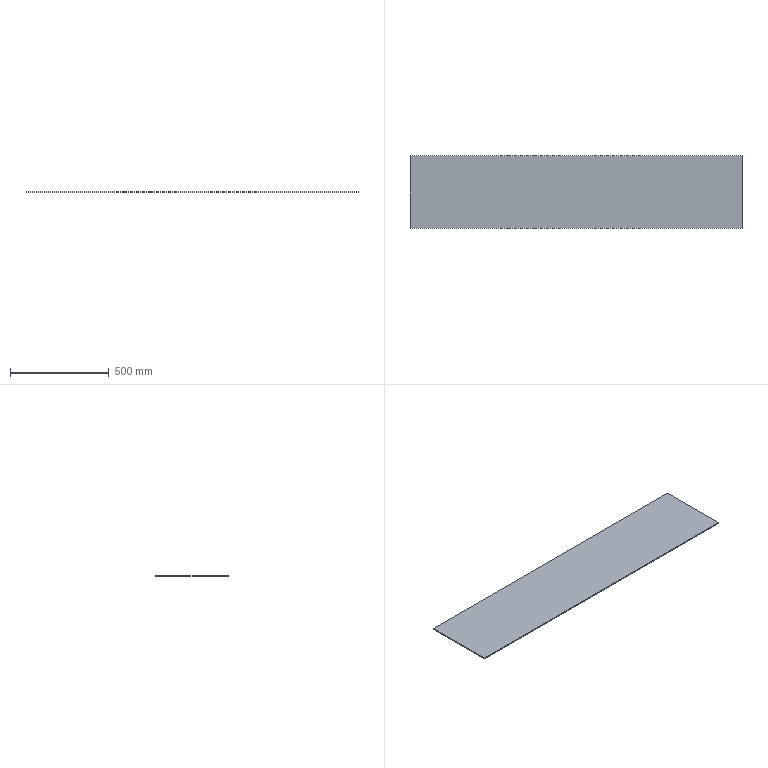Part | SolidWorks | features FlatPattern 1, SMBaseFlange 1, SheetMetal 1 | 1 solid | 6 faces | box 1685 x 367 x 5 mm | volume 3091975 mm3 | plane 6
STEP:
#1=CARTESIAN_POINT('',(842.5,-183.5,0.));
#2=VERTEX_POINT('',#1);
#3=CARTESIAN_POINT('',(842.5,183.5,0.));
#4=VERTEX_POINT('',#3);
#5=CARTESIAN_POINT('',(842.5,183.5,0.));
#6=DIRECTION('',(0.,1.,0.));
#7=VECTOR('',#6,1000.);
#8=LINE('',#5,#7);
#9=EDGE_CURVE('',#2,#4,#8,.T.);
#10=ORIENTED_EDGE('',*,*,#9,.F.);
#11=CARTESIAN_POINT('',(842.5,-183.5,-5.));
#12=VERTEX_POINT('',#11);
#13=CARTESIAN_POINT('',(842.5,-183.5,-5.));
#14=DIRECTION('',(0.,0.,1.));
#15=VECTOR('',#14,1000.);
#16=LINE('',#13,#15);
#17=EDGE_CURVE('',#12,#2,#16,.T.);
#18=ORIENTED_EDGE('',*,*,#17,.F.);
#19=CARTESIAN_POINT('',(842.5,183.5,-5.));
#20=VERTEX_POINT('',#19);
#21=CARTESIAN_POINT('',(842.5,183.5,-5.));
#22=DIRECTION('',(0.,1.,0.));
#23=VECTOR('',#22,1000.);
#24=LINE('',#21,#23);
#25=EDGE_CURVE('',#12,#20,#24,.T.);
#26=ORIENTED_EDGE('',*,*,#25,.T.);
#27=CARTESIAN_POINT('',(842.5,183.5,-5.));
#28=DIRECTION('',(0.,0.,1.));
#29=VECTOR('',#28,1000.);
#30=LINE('',#27,#29);
#31=EDGE_CURVE('',#20,#4,#30,.T.);
#32=ORIENTED_EDGE('',*,*,#31,.T.);
#33=EDGE_LOOP('',(#10,#18,#26,#32));
#34=FACE_OUTER_BOUND('',#33,.T.);
#35=CARTESIAN_POINT('',(842.5,183.5,-5.));
#36=DIRECTION('',(1.,0.,0.));
#37=DIRECTION('',(0.,0.,-1.));
#38=AXIS2_PLACEMENT_3D('',#35,#36,#37);
#39=PLANE('',#38);
#40=ADVANCED_FACE('',(#34),#39,.T.);
#41=CARTESIAN_POINT('',(-842.5,-183.5,0.));
#42=VERTEX_POINT('',#41);
#43=CARTESIAN_POINT('',(-842.5,-183.5,0.));
#44=DIRECTION('',(1.,0.,0.));
#45=VECTOR('',#44,1000.);
#46=LINE('',#43,#45);
#47=EDGE_CURVE('',#42,#2,#46,.T.);
#48=ORIENTED_EDGE('',*,*,#47,.F.);
#49=CARTESIAN_POINT('',(-842.5,-183.5,-5.));
#50=VERTEX_POINT('',#49);
#51=CARTESIAN_POINT('',(-842.5,-183.5,-5.));
#52=DIRECTION('',(0.,0.,1.));
#53=VECTOR('',#52,1000.);
#54=LINE('',#51,#53);
#55=EDGE_CURVE('',#50,#42,#54,.T.);
#56=ORIENTED_EDGE('',*,*,#55,.F.);
#57=CARTESIAN_POINT('',(-842.5,-183.5,-5.));
#58=DIRECTION('',(1.,0.,0.));
#59=VECTOR('',#58,1000.);
#60=LINE('',#57,#59);
#61=EDGE_CURVE('',#50,#12,#60,.T.);
#62=ORIENTED_EDGE('',*,*,#61,.T.);
#63=ORIENTED_EDGE('',*,*,#17,.T.);
#64=EDGE_LOOP('',(#48,#56,#62,#63));
#65=FACE_OUTER_BOUND('',#64,.T.);
#66=CARTESIAN_POINT('',(-842.5,-183.5,-5.));
#67=DIRECTION('',(0.,-1.,0.));
#68=DIRECTION('',(0.,0.,-1.));
#69=AXIS2_PLACEMENT_3D('',#66,#67,#68);
#70=PLANE('',#69);
#71=ADVANCED_FACE('',(#65),#70,.T.);
#72=CARTESIAN_POINT('',(-842.5,183.5,0.));
#73=VERTEX_POINT('',#72);
#74=CARTESIAN_POINT('',(-842.5,183.5,0.));
#75=DIRECTION('',(0.,-1.,0.));
#76=VECTOR('',#75,1000.);
#77=LINE('',#74,#76);
#78=EDGE_CURVE('',#73,#42,#77,.T.);
#79=ORIENTED_EDGE('',*,*,#78,.F.);
#80=CARTESIAN_POINT('',(-842.5,183.5,-5.));
#81=VERTEX_POINT('',#80);
#82=CARTESIAN_POINT('',(-842.5,183.5,-5.));
#83=DIRECTION('',(0.,0.,1.));
#84=VECTOR('',#83,1000.);
#85=LINE('',#82,#84);
#86=EDGE_CURVE('',#81,#73,#85,.T.);
#87=ORIENTED_EDGE('',*,*,#86,.F.);
#88=CARTESIAN_POINT('',(-842.5,183.5,-5.));
#89=DIRECTION('',(0.,-1.,0.));
#90=VECTOR('',#89,1000.);
#91=LINE('',#88,#90);
#92=EDGE_CURVE('',#81,#50,#91,.T.);
#93=ORIENTED_EDGE('',*,*,#92,.T.);
#94=ORIENTED_EDGE('',*,*,#55,.T.);
#95=EDGE_LOOP('',(#79,#87,#93,#94));
#96=FACE_OUTER_BOUND('',#95,.T.);
#97=CARTESIAN_POINT('',(-842.5,183.5,-5.));
#98=DIRECTION('',(-1.,0.,0.));
#99=DIRECTION('',(0.,0.,1.));
#100=AXIS2_PLACEMENT_3D('',#97,#98,#99);
#101=PLANE('',#100);
#102=ADVANCED_FACE('',(#96),#101,.T.);
#103=CARTESIAN_POINT('',(-842.5,183.5,0.));
#104=DIRECTION('',(-1.,0.,0.));
#105=VECTOR('',#104,1000.);
#106=LINE('',#103,#105);
#107=EDGE_CURVE('',#4,#73,#106,.T.);
#108=ORIENTED_EDGE('',*,*,#107,.F.);
#109=ORIENTED_EDGE('',*,*,#31,.F.);
#110=CARTESIAN_POINT('',(-842.5,183.5,-5.));
#111=DIRECTION('',(-1.,0.,0.));
#112=VECTOR('',#111,1000.);
#113=LINE('',#110,#112);
#114=EDGE_CURVE('',#20,#81,#113,.T.);
#115=ORIENTED_EDGE('',*,*,#114,.T.);
#116=ORIENTED_EDGE('',*,*,#86,.T.);
#117=EDGE_LOOP('',(#108,#109,#115,#116));
#118=FACE_OUTER_BOUND('',#117,.T.);
#119=CARTESIAN_POINT('',(-842.5,183.5,-5.));
#120=DIRECTION('',(0.,1.,0.));
#121=DIRECTION('',(0.,0.,1.));
#122=AXIS2_PLACEMENT_3D('',#119,#120,#121);
#123=PLANE('',#122);
#124=ADVANCED_FACE('',(#118),#123,.T.);
#125=ORIENTED_EDGE('',*,*,#25,.F.);
#126=ORIENTED_EDGE('',*,*,#61,.F.);
#127=ORIENTED_EDGE('',*,*,#92,.F.);
#128=ORIENTED_EDGE('',*,*,#114,.F.);
#129=EDGE_LOOP('',(#125,#126,#127,#128));
#130=FACE_OUTER_BOUND('',#129,.T.);
#131=CARTESIAN_POINT('',(842.5,-183.5,-5.));
#132=DIRECTION('',(0.,0.,1.));
#133=DIRECTION('',(1.,0.,0.));
#134=AXIS2_PLACEMENT_3D('',#131,#132,#133);
#135=PLANE('',#134);
#136=ADVANCED_FACE('',(#130),#135,.F.);
#137=ORIENTED_EDGE('',*,*,#9,.T.);
#138=ORIENTED_EDGE('',*,*,#107,.T.);
#139=ORIENTED_EDGE('',*,*,#78,.T.);
#140=ORIENTED_EDGE('',*,*,#47,.T.);
#141=EDGE_LOOP('',(#137,#138,#139,#140));
#142=FACE_OUTER_BOUND('',#141,.T.);
#143=CARTESIAN_POINT('',(842.5,-183.5,0.));
#144=DIRECTION('',(0.,0.,1.));
#145=DIRECTION('',(1.,0.,0.));
#146=AXIS2_PLACEMENT_3D('',#143,#144,#145);
#147=PLANE('',#146);
#148=ADVANCED_FACE('',(#142),#147,.T.);
#149=CLOSED_SHELL('',(#40,#71,#102,#124,#136,#148));
#150=MANIFOLD_SOLID_BREP('',#149);
#151=CARTESIAN_POINT('',(0.,0.,0.));
#152=DIRECTION('',(0.,0.,1.));
#153=DIRECTION('',(1.,0.,0.));
#154=AXIS2_PLACEMENT_3D('',#151,#152,#153);
#155=(LENGTH_UNIT()NAMED_UNIT(*)SI_UNIT(.MILLI.,.METRE.));
#156=UNCERTAINTY_MEASURE_WITH_UNIT(LENGTH_MEASURE(0.00001),#155,'','');
#157=(NAMED_UNIT(*)PLANE_ANGLE_UNIT()SI_UNIT($,.RADIAN.));
#158=(NAMED_UNIT(*)SI_UNIT($,.STERADIAN.)SOLID_ANGLE_UNIT());
#159=(GEOMETRIC_REPRESENTATION_CONTEXT(3)GLOBAL_UNCERTAINTY_ASSIGNED_CONTEXT((#156))GLOBAL_UNIT_ASSIGNED_CONTEXT((#155,#157,#158))REPRESENTATION_CONTEXT('',''));
#160=ADVANCED_BREP_SHAPE_REPRESENTATION('',(#150,#154),#159);